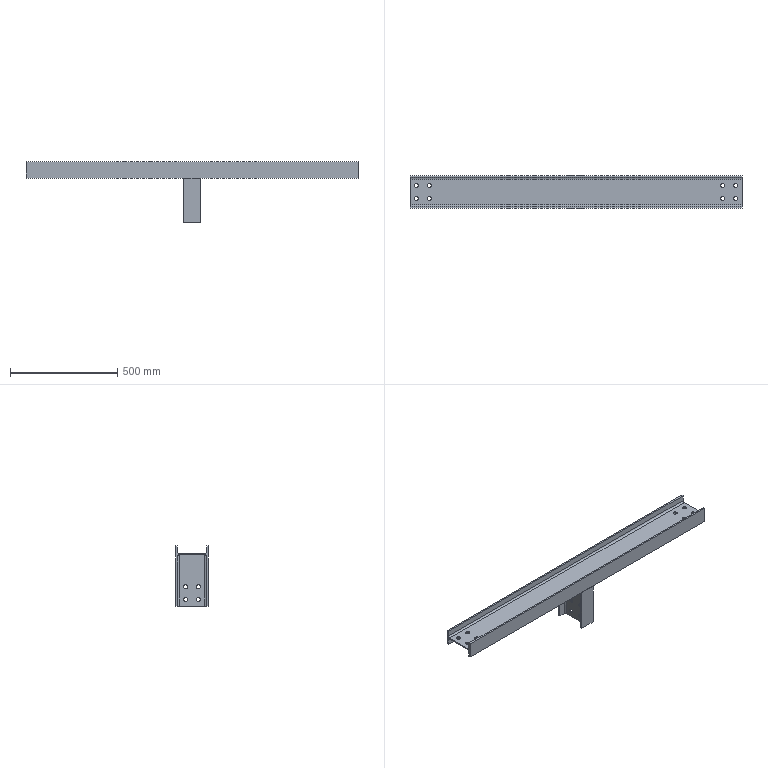Part | STEP file | 粉仓辅梁7主体_Default<As Machined> | 2 solids | 66 faces | box 1545 x 150 x 280 mm | volume 3131691 mm3 | plane 34 | cylinder 32 | commonest cylinder face diameters 19 x24 16 x8